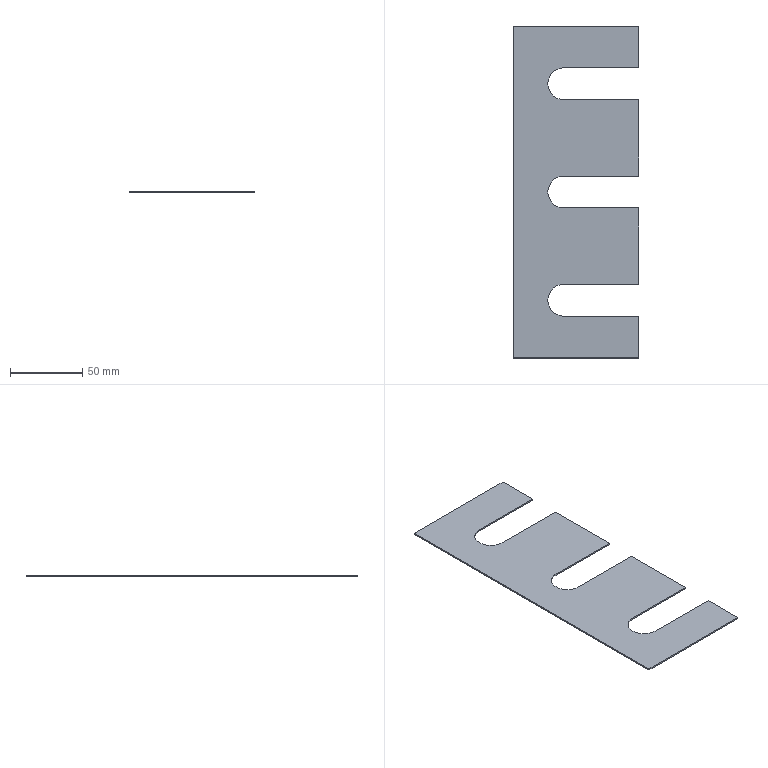Part | STEP file | Adjusting shim 1 | 1 solid | 21 faces | box 87 x 230 x 1 mm | volume 16008 mm3 | plane 15 | cylinder 6 | commonest cylinder face diameters 22 x6